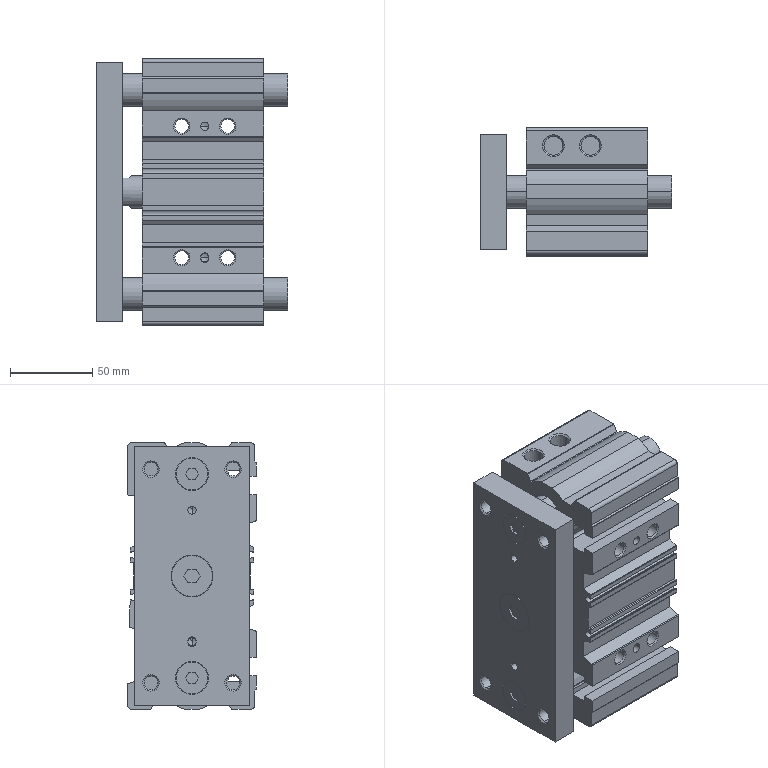Part | 2 solids | 336 faces | box 116.5 x 78 x 162 mm | volume 887155 mm3 | plane 154 | cylinder 134 | cone 48 | commonest cylinder face diameters 8.376 x24 1 x22 5 x20 20 x16 4.2 x12 8.6 x8